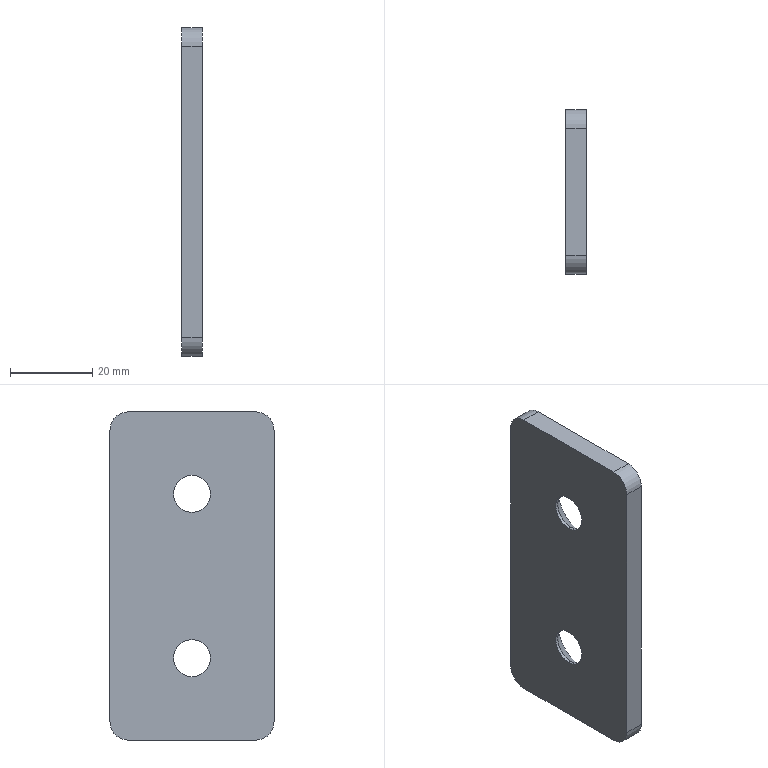Part | SolidWorks | features BaseBody 1 | 1 solid | 18 faces | box 5 x 40 x 80 mm | volume 14588 mm3 | cylinder 8 | plane 6 | cone 4 | commonest cylinder face diameters 9 x8
STEP:
#1=CARTESIAN_POINT('',(5.,20.,35.5));
#2=VERTEX_POINT('',#1);
#3=CARTESIAN_POINT('',(5.,15.5,40.));
#4=VERTEX_POINT('',#3);
#5=CARTESIAN_POINT('',(5.,15.5,35.5));
#6=DIRECTION('',(1.,0.,0.));
#7=DIRECTION('',(0.,0.,-1.));
#8=AXIS2_PLACEMENT_3D('',#5,#6,#7);
#9=CIRCLE('',#8,4.5);
#10=EDGE_CURVE('',#2,#4,#9,.T.);
#11=ORIENTED_EDGE('',*,*,#10,.F.);
#12=CARTESIAN_POINT('',(0.,20.,35.5));
#13=VERTEX_POINT('',#12);
#14=CARTESIAN_POINT('',(5.,20.,35.5));
#15=DIRECTION('',(1.,0.,0.));
#16=VECTOR('',#15,1000.);
#17=LINE('',#14,#16);
#18=EDGE_CURVE('',#13,#2,#17,.T.);
#19=ORIENTED_EDGE('',*,*,#18,.F.);
#20=CARTESIAN_POINT('',(0.,15.5,40.));
#21=VERTEX_POINT('',#20);
#22=CARTESIAN_POINT('',(0.,15.5,35.5));
#23=DIRECTION('',(-1.,0.,0.));
#24=DIRECTION('',(0.,0.,-1.));
#25=AXIS2_PLACEMENT_3D('',#22,#23,#24);
#26=CIRCLE('',#25,4.5);
#27=EDGE_CURVE('',#21,#13,#26,.T.);
#28=ORIENTED_EDGE('',*,*,#27,.F.);
#29=CARTESIAN_POINT('',(5.,15.5,40.));
#30=DIRECTION('',(-1.,0.,0.));
#31=VECTOR('',#30,1000.);
#32=LINE('',#29,#31);
#33=EDGE_CURVE('',#4,#21,#32,.T.);
#34=ORIENTED_EDGE('',*,*,#33,.F.);
#35=EDGE_LOOP('',(#11,#19,#28,#34));
#36=FACE_OUTER_BOUND('',#35,.T.);
#37=CARTESIAN_POINT('',(5.,15.5,35.5));
#38=DIRECTION('',(-1.,0.,0.));
#39=DIRECTION('',(0.,0.,1.));
#40=AXIS2_PLACEMENT_3D('',#37,#38,#39);
#41=CYLINDRICAL_SURFACE('',#40,4.5);
#42=ADVANCED_FACE('',(#36),#41,.T.);
#43=CARTESIAN_POINT('',(5.,15.5,-40.));
#44=VERTEX_POINT('',#43);
#45=CARTESIAN_POINT('',(5.,20.,-35.5));
#46=VERTEX_POINT('',#45);
#47=CARTESIAN_POINT('',(5.,15.5,-35.5));
#48=DIRECTION('',(1.,0.,0.));
#49=DIRECTION('',(0.,0.,-1.));
#50=AXIS2_PLACEMENT_3D('',#47,#48,#49);
#51=CIRCLE('',#50,4.5);
#52=EDGE_CURVE('',#44,#46,#51,.T.);
#53=ORIENTED_EDGE('',*,*,#52,.F.);
#54=CARTESIAN_POINT('',(0.,15.5,-40.));
#55=VERTEX_POINT('',#54);
#56=CARTESIAN_POINT('',(5.,15.5,-40.));
#57=DIRECTION('',(1.,0.,0.));
#58=VECTOR('',#57,1000.);
#59=LINE('',#56,#58);
#60=EDGE_CURVE('',#55,#44,#59,.T.);
#61=ORIENTED_EDGE('',*,*,#60,.F.);
#62=CARTESIAN_POINT('',(0.,20.,-35.5));
#63=VERTEX_POINT('',#62);
#64=CARTESIAN_POINT('',(0.,15.5,-35.5));
#65=DIRECTION('',(-1.,0.,0.));
#66=DIRECTION('',(0.,0.,-1.));
#67=AXIS2_PLACEMENT_3D('',#64,#65,#66);
#68=CIRCLE('',#67,4.5);
#69=EDGE_CURVE('',#63,#55,#68,.T.);
#70=ORIENTED_EDGE('',*,*,#69,.F.);
#71=CARTESIAN_POINT('',(5.,20.,-35.5));
#72=DIRECTION('',(-1.,0.,0.));
#73=VECTOR('',#72,1000.);
#74=LINE('',#71,#73);
#75=EDGE_CURVE('',#46,#63,#74,.T.);
#76=ORIENTED_EDGE('',*,*,#75,.F.);
#77=EDGE_LOOP('',(#53,#61,#70,#76));
#78=FACE_OUTER_BOUND('',#77,.T.);
#79=CARTESIAN_POINT('',(5.,15.5,-35.5));
#80=DIRECTION('',(-1.,0.,0.));
#81=DIRECTION('',(0.,0.,1.));
#82=AXIS2_PLACEMENT_3D('',#79,#80,#81);
#83=CYLINDRICAL_SURFACE('',#82,4.5);
#84=ADVANCED_FACE('',(#78),#83,.T.);
#85=CARTESIAN_POINT('',(5.,-15.5,40.));
#86=VERTEX_POINT('',#85);
#87=CARTESIAN_POINT('',(5.,-20.,35.5));
#88=VERTEX_POINT('',#87);
#89=CARTESIAN_POINT('',(5.,-15.5,35.5));
#90=DIRECTION('',(1.,0.,0.));
#91=DIRECTION('',(0.,0.,-1.));
#92=AXIS2_PLACEMENT_3D('',#89,#90,#91);
#93=CIRCLE('',#92,4.5);
#94=EDGE_CURVE('',#86,#88,#93,.T.);
#95=ORIENTED_EDGE('',*,*,#94,.F.);
#96=CARTESIAN_POINT('',(0.,-15.5,40.));
#97=VERTEX_POINT('',#96);
#98=CARTESIAN_POINT('',(5.,-15.5,40.));
#99=DIRECTION('',(1.,0.,0.));
#100=VECTOR('',#99,1000.);
#101=LINE('',#98,#100);
#102=EDGE_CURVE('',#97,#86,#101,.T.);
#103=ORIENTED_EDGE('',*,*,#102,.F.);
#104=CARTESIAN_POINT('',(0.,-20.,35.5));
#105=VERTEX_POINT('',#104);
#106=CARTESIAN_POINT('',(0.,-15.5,35.5));
#107=DIRECTION('',(-1.,0.,0.));
#108=DIRECTION('',(0.,0.,-1.));
#109=AXIS2_PLACEMENT_3D('',#106,#107,#108);
#110=CIRCLE('',#109,4.5);
#111=EDGE_CURVE('',#105,#97,#110,.T.);
#112=ORIENTED_EDGE('',*,*,#111,.F.);
#113=CARTESIAN_POINT('',(5.,-20.,35.5));
#114=DIRECTION('',(-1.,0.,0.));
#115=VECTOR('',#114,1000.);
#116=LINE('',#113,#115);
#117=EDGE_CURVE('',#88,#105,#116,.T.);
#118=ORIENTED_EDGE('',*,*,#117,.F.);
#119=EDGE_LOOP('',(#95,#103,#112,#118));
#120=FACE_OUTER_BOUND('',#119,.T.);
#121=CARTESIAN_POINT('',(5.,-15.5,35.5));
#122=DIRECTION('',(-1.,0.,0.));
#123=DIRECTION('',(0.,0.,1.));
#124=AXIS2_PLACEMENT_3D('',#121,#122,#123);
#125=CYLINDRICAL_SURFACE('',#124,4.5);
#126=ADVANCED_FACE('',(#120),#125,.T.);
#127=CARTESIAN_POINT('',(5.,-20.,-35.5));
#128=VERTEX_POINT('',#127);
#129=CARTESIAN_POINT('',(5.,-15.5,-40.));
#130=VERTEX_POINT('',#129);
#131=CARTESIAN_POINT('',(5.,-15.5,-35.5));
#132=DIRECTION('',(1.,0.,0.));
#133=DIRECTION('',(0.,0.,-1.));
#134=AXIS2_PLACEMENT_3D('',#131,#132,#133);
#135=CIRCLE('',#134,4.5);
#136=EDGE_CURVE('',#128,#130,#135,.T.);
#137=ORIENTED_EDGE('',*,*,#136,.F.);
#138=CARTESIAN_POINT('',(0.,-20.,-35.5));
#139=VERTEX_POINT('',#138);
#140=CARTESIAN_POINT('',(5.,-20.,-35.5));
#141=DIRECTION('',(1.,0.,0.));
#142=VECTOR('',#141,1000.);
#143=LINE('',#140,#142);
#144=EDGE_CURVE('',#139,#128,#143,.T.);
#145=ORIENTED_EDGE('',*,*,#144,.F.);
#146=CARTESIAN_POINT('',(0.,-15.5,-40.));
#147=VERTEX_POINT('',#146);
#148=CARTESIAN_POINT('',(0.,-15.5,-35.5));
#149=DIRECTION('',(-1.,0.,0.));
#150=DIRECTION('',(0.,0.,-1.));
#151=AXIS2_PLACEMENT_3D('',#148,#149,#150);
#152=CIRCLE('',#151,4.5);
#153=EDGE_CURVE('',#147,#139,#152,.T.);
#154=ORIENTED_EDGE('',*,*,#153,.F.);
#155=CARTESIAN_POINT('',(5.,-15.5,-40.));
#156=DIRECTION('',(-1.,0.,0.));
#157=VECTOR('',#156,1000.);
#158=LINE('',#155,#157);
#159=EDGE_CURVE('',#130,#147,#158,.T.);
#160=ORIENTED_EDGE('',*,*,#159,.F.);
#161=EDGE_LOOP('',(#137,#145,#154,#160));
#162=FACE_OUTER_BOUND('',#161,.T.);
#163=CARTESIAN_POINT('',(5.,-15.5,-35.5));
#164=DIRECTION('',(-1.,0.,0.));
#165=DIRECTION('',(0.,0.,1.));
#166=AXIS2_PLACEMENT_3D('',#163,#164,#165);
#167=CYLINDRICAL_SURFACE('',#166,4.5);
#168=ADVANCED_FACE('',(#162),#167,.T.);
#169=CARTESIAN_POINT('',(0.7,0.,24.5));
#170=VERTEX_POINT('',#169);
#171=CARTESIAN_POINT('',(5.,0.,28.8));
#172=VERTEX_POINT('',#171);
#173=CARTESIAN_POINT('',(5.,0.,28.8));
#174=DIRECTION('',(0.7071,0.,0.7071));
#175=VECTOR('',#174,1000.);
#176=LINE('',#173,#175);
#177=EDGE_CURVE('',#170,#172,#176,.T.);
#178=ORIENTED_EDGE('',*,*,#177,.F.);
#179=CARTESIAN_POINT('',(0.7,0.,15.5));
#180=VERTEX_POINT('',#179);
#181=CARTESIAN_POINT('',(0.7,0.,20.));
#182=DIRECTION('',(1.,0.,0.));
#183=DIRECTION('',(0.,0.,-1.));
#184=AXIS2_PLACEMENT_3D('',#181,#182,#183);
#185=CIRCLE('',#184,4.5);
#186=EDGE_CURVE('',#180,#170,#185,.T.);
#187=ORIENTED_EDGE('',*,*,#186,.F.);
#188=CARTESIAN_POINT('',(5.,0.,11.2));
#189=VERTEX_POINT('',#188);
#190=CARTESIAN_POINT('',(5.,0.,11.2));
#191=DIRECTION('',(0.7071,0.,-0.7071));
#192=VECTOR('',#191,1000.);
#193=LINE('',#190,#192);
#194=EDGE_CURVE('',#180,#189,#193,.T.);
#195=ORIENTED_EDGE('',*,*,#194,.T.);
#196=CARTESIAN_POINT('',(5.,0.,20.));
#197=DIRECTION('',(1.,0.,0.));
#198=DIRECTION('',(0.,0.,-1.));
#199=AXIS2_PLACEMENT_3D('',#196,#197,#198);
#200=CIRCLE('',#199,8.8);
#201=EDGE_CURVE('',#189,#172,#200,.T.);
#202=ORIENTED_EDGE('',*,*,#201,.T.);
#203=EDGE_LOOP('',(#178,#187,#195,#202));
#204=FACE_OUTER_BOUND('',#203,.T.);
#205=CARTESIAN_POINT('',(5.,0.,20.));
#206=DIRECTION('',(1.,0.,0.));
#207=DIRECTION('',(0.,0.,-1.));
#208=AXIS2_PLACEMENT_3D('',#205,#206,#207);
#209=CONICAL_SURFACE('',#208,8.8,0.7854);
#210=ADVANCED_FACE('',(#204),#209,.F.);
#211=CARTESIAN_POINT('',(0.,0.,24.5));
#212=VERTEX_POINT('',#211);
#213=CARTESIAN_POINT('',(5.,0.,24.5));
#214=DIRECTION('',(1.,0.,0.));
#215=VECTOR('',#214,1000.);
#216=LINE('',#213,#215);
#217=EDGE_CURVE('',#212,#170,#216,.T.);
#218=ORIENTED_EDGE('',*,*,#217,.F.);
#219=CARTESIAN_POINT('',(0.,0.,15.5));
#220=VERTEX_POINT('',#219);
#221=CARTESIAN_POINT('',(0.,0.,20.));
#222=DIRECTION('',(1.,0.,0.));
#223=DIRECTION('',(0.,0.,-1.));
#224=AXIS2_PLACEMENT_3D('',#221,#222,#223);
#225=CIRCLE('',#224,4.5);
#226=EDGE_CURVE('',#220,#212,#225,.T.);
#227=ORIENTED_EDGE('',*,*,#226,.F.);
#228=CARTESIAN_POINT('',(5.,0.,15.5));
#229=DIRECTION('',(1.,0.,0.));
#230=VECTOR('',#229,1000.);
#231=LINE('',#228,#230);
#232=EDGE_CURVE('',#220,#180,#231,.T.);
#233=ORIENTED_EDGE('',*,*,#232,.T.);
#234=ORIENTED_EDGE('',*,*,#186,.T.);
#235=EDGE_LOOP('',(#218,#227,#233,#234));
#236=FACE_OUTER_BOUND('',#235,.T.);
#237=CARTESIAN_POINT('',(5.,0.,20.));
#238=DIRECTION('',(1.,0.,0.));
#239=DIRECTION('',(0.,0.,-1.));
#240=AXIS2_PLACEMENT_3D('',#237,#238,#239);
#241=CYLINDRICAL_SURFACE('',#240,4.5);
#242=ADVANCED_FACE('',(#236),#241,.F.);
#243=CARTESIAN_POINT('',(0.7,0.,-15.5));
#244=VERTEX_POINT('',#243);
#245=CARTESIAN_POINT('',(5.,0.,-11.2));
#246=VERTEX_POINT('',#245);
#247=CARTESIAN_POINT('',(5.,0.,-11.2));
#248=DIRECTION('',(0.7071,0.,0.7071));
#249=VECTOR('',#248,1000.);
#250=LINE('',#247,#249);
#251=EDGE_CURVE('',#244,#246,#250,.T.);
#252=ORIENTED_EDGE('',*,*,#251,.F.);
#253=CARTESIAN_POINT('',(0.7,0.,-24.5));
#254=VERTEX_POINT('',#253);
#255=CARTESIAN_POINT('',(0.7,0.,-20.));
#256=DIRECTION('',(1.,0.,0.));
#257=DIRECTION('',(0.,0.,-1.));
#258=AXIS2_PLACEMENT_3D('',#255,#256,#257);
#259=CIRCLE('',#258,4.5);
#260=EDGE_CURVE('',#254,#244,#259,.T.);
#261=ORIENTED_EDGE('',*,*,#260,.F.);
#262=CARTESIAN_POINT('',(5.,0.,-28.8));
#263=VERTEX_POINT('',#262);
#264=CARTESIAN_POINT('',(5.,0.,-28.8));
#265=DIRECTION('',(0.7071,0.,-0.7071));
#266=VECTOR('',#265,1000.);
#267=LINE('',#264,#266);
#268=EDGE_CURVE('',#254,#263,#267,.T.);
#269=ORIENTED_EDGE('',*,*,#268,.T.);
#270=CARTESIAN_POINT('',(5.,0.,-20.));
#271=DIRECTION('',(1.,0.,0.));
#272=DIRECTION('',(0.,0.,-1.));
#273=AXIS2_PLACEMENT_3D('',#270,#271,#272);
#274=CIRCLE('',#273,8.8);
#275=EDGE_CURVE('',#263,#246,#274,.T.);
#276=ORIENTED_EDGE('',*,*,#275,.T.);
#277=EDGE_LOOP('',(#252,#261,#269,#276));
#278=FACE_OUTER_BOUND('',#277,.T.);
#279=CARTESIAN_POINT('',(5.,0.,-20.));
#280=DIRECTION('',(1.,0.,0.));
#281=DIRECTION('',(0.,0.,-1.));
#282=AXIS2_PLACEMENT_3D('',#279,#280,#281);
#283=CONICAL_SURFACE('',#282,8.8,0.7854);
#284=ADVANCED_FACE('',(#278),#283,.F.);
#285=CARTESIAN_POINT('',(0.,0.,-15.5));
#286=VERTEX_POINT('',#285);
#287=CARTESIAN_POINT('',(5.,0.,-15.5));
#288=DIRECTION('',(1.,0.,0.));
#289=VECTOR('',#288,1000.);
#290=LINE('',#287,#289);
#291=EDGE_CURVE('',#286,#244,#290,.T.);
#292=ORIENTED_EDGE('',*,*,#291,.F.);
#293=CARTESIAN_POINT('',(0.,0.,-24.5));
#294=VERTEX_POINT('',#293);
#295=CARTESIAN_POINT('',(0.,0.,-20.));
#296=DIRECTION('',(1.,0.,0.));
#297=DIRECTION('',(0.,0.,-1.));
#298=AXIS2_PLACEMENT_3D('',#295,#296,#297);
#299=CIRCLE('',#298,4.5);
#300=EDGE_CURVE('',#294,#286,#299,.T.);
#301=ORIENTED_EDGE('',*,*,#300,.F.);
#302=CARTESIAN_POINT('',(5.,0.,-24.5));
#303=DIRECTION('',(1.,0.,0.));
#304=VECTOR('',#303,1000.);
#305=LINE('',#302,#304);
#306=EDGE_CURVE('',#294,#254,#305,.T.);
#307=ORIENTED_EDGE('',*,*,#306,.T.);
#308=ORIENTED_EDGE('',*,*,#260,.T.);
#309=EDGE_LOOP('',(#292,#301,#307,#308));
#310=FACE_OUTER_BOUND('',#309,.T.);
#311=CARTESIAN_POINT('',(5.,0.,-20.));
#312=DIRECTION('',(1.,0.,0.));
#313=DIRECTION('',(0.,0.,-1.));
#314=AXIS2_PLACEMENT_3D('',#311,#312,#313);
#315=CYLINDRICAL_SURFACE('',#314,4.5);
#316=ADVANCED_FACE('',(#310),#315,.F.);
#317=ORIENTED_EDGE('',*,*,#300,.T.);
#318=CARTESIAN_POINT('',(0.,0.,-20.));
#319=DIRECTION('',(1.,0.,0.));
#320=DIRECTION('',(0.,0.,-1.));
#321=AXIS2_PLACEMENT_3D('',#318,#319,#320);
#322=CIRCLE('',#321,4.5);
#323=EDGE_CURVE('',#286,#294,#322,.T.);
#324=ORIENTED_EDGE('',*,*,#323,.T.);
#325=EDGE_LOOP('',(#317,#324));
#326=FACE_BOUND('',#325,.T.);
#327=ORIENTED_EDGE('',*,*,#226,.T.);
#328=CARTESIAN_POINT('',(0.,0.,20.));
#329=DIRECTION('',(1.,0.,0.));
#330=DIRECTION('',(0.,0.,-1.));
#331=AXIS2_PLACEMENT_3D('',#328,#329,#330);
#332=CIRCLE('',#331,4.5);
#333=EDGE_CURVE('',#212,#220,#332,.T.);
#334=ORIENTED_EDGE('',*,*,#333,.T.);
#335=EDGE_LOOP('',(#327,#334));
#336=FACE_BOUND('',#335,.T.);
#337=CARTESIAN_POINT('',(0.,20.,-40.));
#338=DIRECTION('',(0.,1.,0.));
#339=VECTOR('',#338,1000.);
#340=LINE('',#337,#339);
#341=EDGE_CURVE('',#147,#55,#340,.T.);
#342=ORIENTED_EDGE('',*,*,#341,.F.);
#343=ORIENTED_EDGE('',*,*,#153,.T.);
#344=CARTESIAN_POINT('',(0.,-20.,40.));
#345=DIRECTION('',(0.,0.,-1.));
#346=VECTOR('',#345,1000.);
#347=LINE('',#344,#346);
#348=EDGE_CURVE('',#105,#139,#347,.T.);
#349=ORIENTED_EDGE('',*,*,#348,.F.);
#350=ORIENTED_EDGE('',*,*,#111,.T.);
#351=CARTESIAN_POINT('',(0.,20.,40.));
#352=DIRECTION('',(0.,-1.,0.));
#353=VECTOR('',#352,1000.);
#354=LINE('',#351,#353);
#355=EDGE_CURVE('',#21,#97,#354,.T.);
#356=ORIENTED_EDGE('',*,*,#355,.F.);
#357=ORIENTED_EDGE('',*,*,#27,.T.);
#358=CARTESIAN_POINT('',(0.,20.,40.));
#359=DIRECTION('',(0.,0.,1.));
#360=VECTOR('',#359,1000.);
#361=LINE('',#358,#360);
#362=EDGE_CURVE('',#63,#13,#361,.T.);
#363=ORIENTED_EDGE('',*,*,#362,.F.);
#364=ORIENTED_EDGE('',*,*,#69,.T.);
#365=EDGE_LOOP('',(#342,#343,#349,#350,#356,#357,#363,#364));
#366=FACE_OUTER_BOUND('',#365,.T.);
#367=CARTESIAN_POINT('',(0.,0.,0.));
#368=DIRECTION('',(1.,0.,0.));
#369=DIRECTION('',(0.,1.,0.));
#370=AXIS2_PLACEMENT_3D('',#367,#368,#369);
#371=PLANE('',#370);
#372=ADVANCED_FACE('',(#326,#336,#366),#371,.F.);
#373=ORIENTED_EDGE('',*,*,#275,.F.);
#374=CARTESIAN_POINT('',(5.,0.,-20.));
#375=DIRECTION('',(1.,0.,0.));
#376=DIRECTION('',(0.,0.,-1.));
#377=AXIS2_PLACEMENT_3D('',#374,#375,#376);
#378=CIRCLE('',#377,8.8);
#379=EDGE_CURVE('',#246,#263,#378,.T.);
#380=ORIENTED_EDGE('',*,*,#379,.F.);
#381=EDGE_LOOP('',(#373,#380));
#382=FACE_BOUND('',#381,.T.);
#383=ORIENTED_EDGE('',*,*,#201,.F.);
#384=CARTESIAN_POINT('',(5.,0.,20.));
#385=DIRECTION('',(1.,0.,0.));
#386=DIRECTION('',(0.,0.,-1.));
#387=AXIS2_PLACEMENT_3D('',#384,#385,#386);
#388=CIRCLE('',#387,8.8);
#389=EDGE_CURVE('',#172,#189,#388,.T.);
#390=ORIENTED_EDGE('',*,*,#389,.F.);
#391=EDGE_LOOP('',(#383,#390));
#392=FACE_BOUND('',#391,.T.);
#393=CARTESIAN_POINT('',(5.,-20.,40.));
#394=DIRECTION('',(0.,0.,-1.));
#395=VECTOR('',#394,1000.);
#396=LINE('',#393,#395);
#397=EDGE_CURVE('',#88,#128,#396,.T.);
#398=ORIENTED_EDGE('',*,*,#397,.T.);
#399=ORIENTED_EDGE('',*,*,#136,.T.);
#400=CARTESIAN_POINT('',(5.,20.,-40.));
#401=DIRECTION('',(0.,1.,0.));
#402=VECTOR('',#401,1000.);
#403=LINE('',#400,#402);
#404=EDGE_CURVE('',#130,#44,#403,.T.);
#405=ORIENTED_EDGE('',*,*,#404,.T.);
#406=ORIENTED_EDGE('',*,*,#52,.T.);
#407=CARTESIAN_POINT('',(5.,20.,40.));
#408=DIRECTION('',(0.,0.,1.));
#409=VECTOR('',#408,1000.);
#410=LINE('',#407,#409);
#411=EDGE_CURVE('',#46,#2,#410,.T.);
#412=ORIENTED_EDGE('',*,*,#411,.T.);
#413=ORIENTED_EDGE('',*,*,#10,.T.);
#414=CARTESIAN_POINT('',(5.,20.,40.));
#415=DIRECTION('',(0.,-1.,0.));
#416=VECTOR('',#415,1000.);
#417=LINE('',#414,#416);
#418=EDGE_CURVE('',#4,#86,#417,.T.);
#419=ORIENTED_EDGE('',*,*,#418,.T.);
#420=ORIENTED_EDGE('',*,*,#94,.T.);
#421=EDGE_LOOP('',(#398,#399,#405,#406,#412,#413,#419,#420));
#422=FACE_OUTER_BOUND('',#421,.T.);
#423=CARTESIAN_POINT('',(5.,0.,0.));
#424=DIRECTION('',(1.,0.,0.));
#425=DIRECTION('',(0.,1.,0.));
#426=AXIS2_PLACEMENT_3D('',#423,#424,#425);
#427=PLANE('',#426);
#428=ADVANCED_FACE('',(#382,#392,#422),#427,.T.);
#429=ORIENTED_EDGE('',*,*,#348,.T.);
#430=ORIENTED_EDGE('',*,*,#144,.T.);
#431=ORIENTED_EDGE('',*,*,#397,.F.);
#432=ORIENTED_EDGE('',*,*,#117,.T.);
#433=EDGE_LOOP('',(#429,#430,#431,#432));
#434=FACE_OUTER_BOUND('',#433,.T.);
#435=CARTESIAN_POINT('',(5.,-20.,40.));
#436=DIRECTION('',(0.,1.,0.));
#437=DIRECTION('',(1.,0.,0.));
#438=AXIS2_PLACEMENT_3D('',#435,#436,#437);
#439=PLANE('',#438);
#440=ADVANCED_FACE('',(#434),#439,.F.);
#441=ORIENTED_EDGE('',*,*,#355,.T.);
#442=ORIENTED_EDGE('',*,*,#102,.T.);
#443=ORIENTED_EDGE('',*,*,#418,.F.);
#444=ORIENTED_EDGE('',*,*,#33,.T.);
#445=EDGE_LOOP('',(#441,#442,#443,#444));
#446=FACE_OUTER_BOUND('',#445,.T.);
#447=CARTESIAN_POINT('',(5.,20.,40.));
#448=DIRECTION('',(0.,0.,-1.));
#449=DIRECTION('',(0.,-1.,0.));
#450=AXIS2_PLACEMENT_3D('',#447,#448,#449);
#451=PLANE('',#450);
#452=ADVANCED_FACE('',(#446),#451,.F.);
#453=ORIENTED_EDGE('',*,*,#411,.F.);
#454=ORIENTED_EDGE('',*,*,#75,.T.);
#455=ORIENTED_EDGE('',*,*,#362,.T.);
#456=ORIENTED_EDGE('',*,*,#18,.T.);
#457=EDGE_LOOP('',(#453,#454,#455,#456));
#458=FACE_OUTER_BOUND('',#457,.T.);
#459=CARTESIAN_POINT('',(5.,20.,40.));
#460=DIRECTION('',(0.,-1.,0.));
#461=DIRECTION('',(0.,0.,-1.));
#462=AXIS2_PLACEMENT_3D('',#459,#460,#461);
#463=PLANE('',#462);
#464=ADVANCED_FACE('',(#458),#463,.F.);
#465=ORIENTED_EDGE('',*,*,#404,.F.);
#466=ORIENTED_EDGE('',*,*,#159,.T.);
#467=ORIENTED_EDGE('',*,*,#341,.T.);
#468=ORIENTED_EDGE('',*,*,#60,.T.);
#469=EDGE_LOOP('',(#465,#466,#467,#468));
#470=FACE_OUTER_BOUND('',#469,.T.);
#471=CARTESIAN_POINT('',(5.,20.,-40.));
#472=DIRECTION('',(0.,0.,1.));
#473=DIRECTION('',(1.,0.,0.));
#474=AXIS2_PLACEMENT_3D('',#471,#472,#473);
#475=PLANE('',#474);
#476=ADVANCED_FACE('',(#470),#475,.F.);
#477=ORIENTED_EDGE('',*,*,#323,.F.);
#478=ORIENTED_EDGE('',*,*,#291,.T.);
#479=CARTESIAN_POINT('',(0.7,0.,-20.));
#480=DIRECTION('',(1.,0.,0.));
#481=DIRECTION('',(0.,0.,-1.));
#482=AXIS2_PLACEMENT_3D('',#479,#480,#481);
#483=CIRCLE('',#482,4.5);
#484=EDGE_CURVE('',#244,#254,#483,.T.);
#485=ORIENTED_EDGE('',*,*,#484,.T.);
#486=ORIENTED_EDGE('',*,*,#306,.F.);
#487=EDGE_LOOP('',(#477,#478,#485,#486));
#488=FACE_OUTER_BOUND('',#487,.T.);
#489=CARTESIAN_POINT('',(5.,0.,-20.));
#490=DIRECTION('',(1.,0.,0.));
#491=DIRECTION('',(0.,0.,-1.));
#492=AXIS2_PLACEMENT_3D('',#489,#490,#491);
#493=CYLINDRICAL_SURFACE('',#492,4.5);
#494=ADVANCED_FACE('',(#488),#493,.F.);
#495=ORIENTED_EDGE('',*,*,#484,.F.);
#496=ORIENTED_EDGE('',*,*,#251,.T.);
#497=ORIENTED_EDGE('',*,*,#379,.T.);
#498=ORIENTED_EDGE('',*,*,#268,.F.);
#499=EDGE_LOOP('',(#495,#496,#497,#498));
#500=FACE_OUTER_BOUND('',#499,.T.);
#501=CARTESIAN_POINT('',(5.,0.,-20.));
#502=DIRECTION('',(1.,0.,0.));
#503=DIRECTION('',(0.,0.,-1.));
#504=AXIS2_PLACEMENT_3D('',#501,#502,#503);
#505=CONICAL_SURFACE('',#504,8.8,0.7854);
#506=ADVANCED_FACE('',(#500),#505,.F.);
#507=ORIENTED_EDGE('',*,*,#333,.F.);
#508=ORIENTED_EDGE('',*,*,#217,.T.);
#509=CARTESIAN_POINT('',(0.7,0.,20.));
#510=DIRECTION('',(1.,0.,0.));
#511=DIRECTION('',(0.,0.,-1.));
#512=AXIS2_PLACEMENT_3D('',#509,#510,#511);
#513=CIRCLE('',#512,4.5);
#514=EDGE_CURVE('',#170,#180,#513,.T.);
#515=ORIENTED_EDGE('',*,*,#514,.T.);
#516=ORIENTED_EDGE('',*,*,#232,.F.);
#517=EDGE_LOOP('',(#507,#508,#515,#516));
#518=FACE_OUTER_BOUND('',#517,.T.);
#519=CARTESIAN_POINT('',(5.,0.,20.));
#520=DIRECTION('',(1.,0.,0.));
#521=DIRECTION('',(0.,0.,-1.));
#522=AXIS2_PLACEMENT_3D('',#519,#520,#521);
#523=CYLINDRICAL_SURFACE('',#522,4.5);
#524=ADVANCED_FACE('',(#518),#523,.F.);
#525=ORIENTED_EDGE('',*,*,#514,.F.);
#526=ORIENTED_EDGE('',*,*,#177,.T.);
#527=ORIENTED_EDGE('',*,*,#389,.T.);
#528=ORIENTED_EDGE('',*,*,#194,.F.);
#529=EDGE_LOOP('',(#525,#526,#527,#528));
#530=FACE_OUTER_BOUND('',#529,.T.);
#531=CARTESIAN_POINT('',(5.,0.,20.));
#532=DIRECTION('',(1.,0.,0.));
#533=DIRECTION('',(0.,0.,-1.));
#534=AXIS2_PLACEMENT_3D('',#531,#532,#533);
#535=CONICAL_SURFACE('',#534,8.8,0.7854);
#536=ADVANCED_FACE('',(#530),#535,.F.);
#537=CLOSED_SHELL('',(#42,#84,#126,#168,#210,#242,#284,#316,#372,#428,#440,#452,#464,#476,#494,#506,#524,#536));
#538=MANIFOLD_SOLID_BREP('',#537);
#539=CARTESIAN_POINT('',(0.,0.,0.));
#540=DIRECTION('',(0.,0.,1.));
#541=DIRECTION('',(1.,0.,0.));
#542=AXIS2_PLACEMENT_3D('',#539,#540,#541);
#543=(LENGTH_UNIT()NAMED_UNIT(*)SI_UNIT(.MILLI.,.METRE.));
#544=UNCERTAINTY_MEASURE_WITH_UNIT(LENGTH_MEASURE(0.00001),#543,'','');
#545=(NAMED_UNIT(*)PLANE_ANGLE_UNIT()SI_UNIT($,.RADIAN.));
#546=(NAMED_UNIT(*)SI_UNIT($,.STERADIAN.)SOLID_ANGLE_UNIT());
#547=(GEOMETRIC_REPRESENTATION_CONTEXT(3)GLOBAL_UNCERTAINTY_ASSIGNED_CONTEXT((#544))GLOBAL_UNIT_ASSIGNED_CONTEXT((#543,#545,#546))REPRESENTATION_CONTEXT('',''));
#548=ADVANCED_BREP_SHAPE_REPRESENTATION('',(#538,#542),#547);